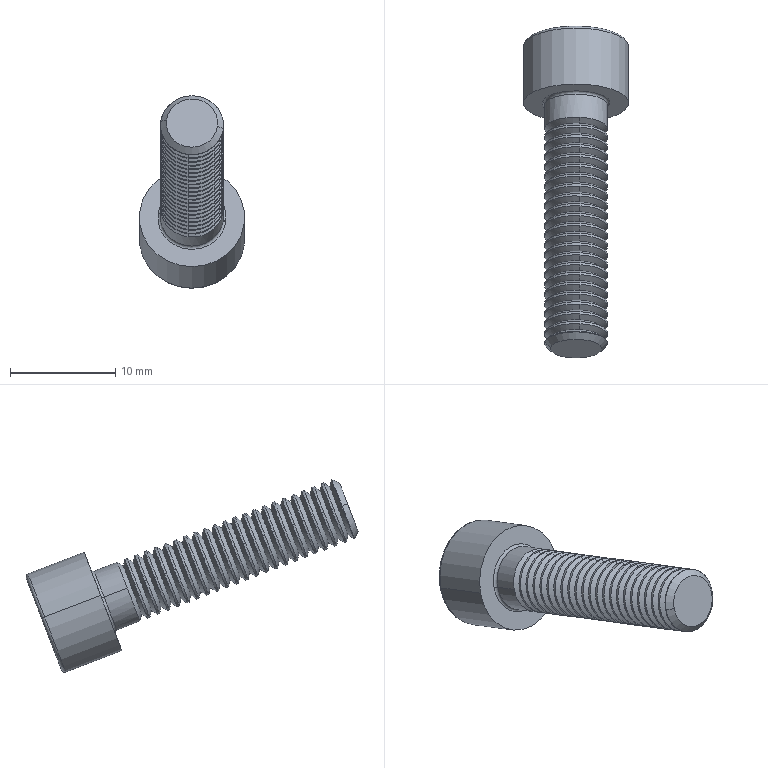Part | STEP file | Socket Head Cap Screw_ISO(ISO 4762 M6 x 25 --- 25S)_Valor predeterminado | 1 solid | 159 faces | box 10 x 31.522 x 18.292 mm | volume 1014 mm3 | cone 92 | cylinder 48 | plane 15 | torus 4 | commonest cylinder face diameters 6 x46 10 x2